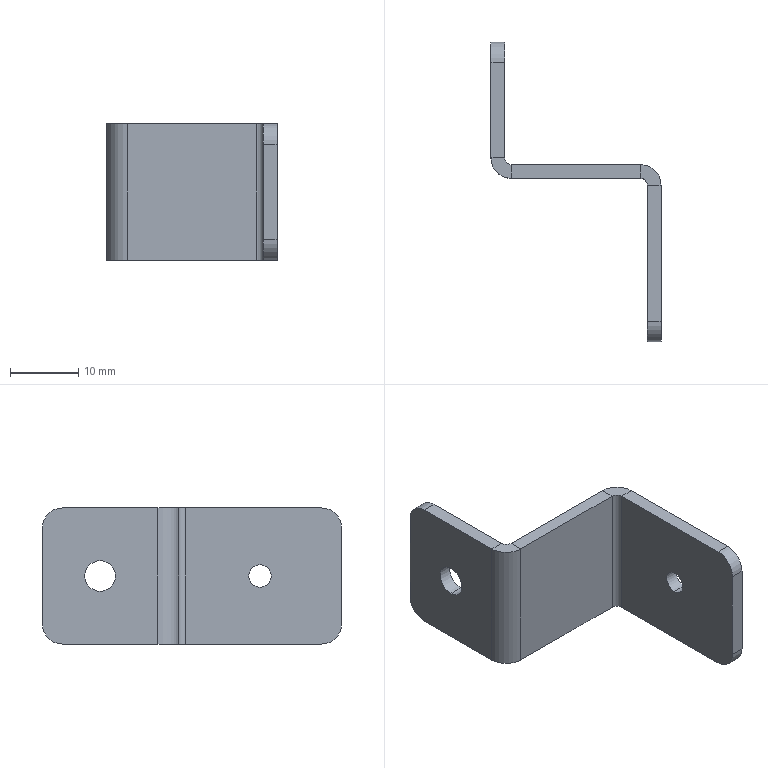Part | NX | features BREP 1 | 1 solid | 30 faces | box 25 x 44 x 20 mm | volume 2547 mm3 | plane 18 | cylinder 12 | commonest cylinder face diameters 6 x6 2 x2 3.3 x2 4.5 x2
STEP:
#1=CARTESIAN_POINT('',(23.,-12.,1.65));
#2=VERTEX_POINT('',#1);
#3=CARTESIAN_POINT('',(25.,-12.,1.65));
#4=VERTEX_POINT('',#3);
#5=CARTESIAN_POINT('',(25.,-12.,1.65));
#6=DIRECTION('',(1.,0.,0.));
#7=VECTOR('',#6,1000.);
#8=LINE('',#5,#7);
#9=EDGE_CURVE('',#2,#4,#8,.T.);
#10=ORIENTED_EDGE('',*,*,#9,.F.);
#11=CARTESIAN_POINT('',(23.,-12.,-1.65));
#12=VERTEX_POINT('',#11);
#13=CARTESIAN_POINT('',(23.,-12.,0.));
#14=DIRECTION('',(-1.,0.,0.));
#15=DIRECTION('',(0.,-1.,0.));
#16=AXIS2_PLACEMENT_3D('',#13,#14,#15);
#17=CIRCLE('',#16,1.65);
#18=EDGE_CURVE('',#2,#12,#17,.T.);
#19=ORIENTED_EDGE('',*,*,#18,.T.);
#20=CARTESIAN_POINT('',(25.,-12.,-1.65));
#21=VERTEX_POINT('',#20);
#22=CARTESIAN_POINT('',(25.,-12.,-1.65));
#23=DIRECTION('',(1.,0.,0.));
#24=VECTOR('',#23,1000.);
#25=LINE('',#22,#24);
#26=EDGE_CURVE('',#12,#21,#25,.T.);
#27=ORIENTED_EDGE('',*,*,#26,.T.);
#28=CARTESIAN_POINT('',(25.,-12.,0.));
#29=DIRECTION('',(1.,0.,0.));
#30=DIRECTION('',(0.,0.,-1.));
#31=AXIS2_PLACEMENT_3D('',#28,#29,#30);
#32=CIRCLE('',#31,1.65);
#33=EDGE_CURVE('',#21,#4,#32,.T.);
#34=ORIENTED_EDGE('',*,*,#33,.T.);
#35=EDGE_LOOP('',(#10,#19,#27,#34));
#36=FACE_BOUND('',#35,.T.);
#37=CARTESIAN_POINT('',(25.,-12.,0.));
#38=DIRECTION('',(1.,0.,0.));
#39=DIRECTION('',(0.,0.,-1.));
#40=AXIS2_PLACEMENT_3D('',#37,#38,#39);
#41=CYLINDRICAL_SURFACE('',#40,1.65);
#42=ADVANCED_FACE('',(#36),#41,.F.);
#43=CARTESIAN_POINT('',(0.,11.5,-2.25));
#44=VERTEX_POINT('',#43);
#45=CARTESIAN_POINT('',(2.,11.5,-2.25));
#46=VERTEX_POINT('',#45);
#47=CARTESIAN_POINT('',(0.,11.5,-2.25));
#48=DIRECTION('',(-1.,0.,0.));
#49=VECTOR('',#48,1000.);
#50=LINE('',#47,#49);
#51=EDGE_CURVE('',#44,#46,#50,.F.);
#52=ORIENTED_EDGE('',*,*,#51,.T.);
#53=CARTESIAN_POINT('',(2.,11.5,2.25));
#54=VERTEX_POINT('',#53);
#55=CARTESIAN_POINT('',(2.,11.5,0.));
#56=DIRECTION('',(-1.,0.,0.));
#57=DIRECTION('',(0.,0.,1.));
#58=AXIS2_PLACEMENT_3D('',#55,#56,#57);
#59=CIRCLE('',#58,2.25);
#60=EDGE_CURVE('',#54,#46,#59,.T.);
#61=ORIENTED_EDGE('',*,*,#60,.F.);
#62=CARTESIAN_POINT('',(0.,11.5,2.25));
#63=VERTEX_POINT('',#62);
#64=CARTESIAN_POINT('',(0.,11.5,2.25));
#65=DIRECTION('',(-1.,0.,0.));
#66=VECTOR('',#65,1000.);
#67=LINE('',#64,#66);
#68=EDGE_CURVE('',#63,#54,#67,.F.);
#69=ORIENTED_EDGE('',*,*,#68,.F.);
#70=CARTESIAN_POINT('',(0.,11.5,0.));
#71=DIRECTION('',(-1.,0.,0.));
#72=DIRECTION('',(0.,0.,1.));
#73=AXIS2_PLACEMENT_3D('',#70,#71,#72);
#74=CIRCLE('',#73,2.25);
#75=EDGE_CURVE('',#63,#44,#74,.T.);
#76=ORIENTED_EDGE('',*,*,#75,.T.);
#77=EDGE_LOOP('',(#52,#61,#69,#76));
#78=FACE_BOUND('',#77,.T.);
#79=CARTESIAN_POINT('',(0.,11.5,0.));
#80=DIRECTION('',(-1.,0.,0.));
#81=DIRECTION('',(0.,0.,1.));
#82=AXIS2_PLACEMENT_3D('',#79,#80,#81);
#83=CYLINDRICAL_SURFACE('',#82,2.25);
#84=ADVANCED_FACE('',(#78),#83,.F.);
#85=CARTESIAN_POINT('',(25.,-24.,-7.));
#86=VERTEX_POINT('',#85);
#87=CARTESIAN_POINT('',(25.,-21.,-10.));
#88=VERTEX_POINT('',#87);
#89=CARTESIAN_POINT('',(25.,-21.,-7.));
#90=DIRECTION('',(1.,0.,0.));
#91=DIRECTION('',(0.,-1.,0.));
#92=AXIS2_PLACEMENT_3D('',#89,#90,#91);
#93=CIRCLE('',#92,3.);
#94=EDGE_CURVE('',#86,#88,#93,.T.);
#95=ORIENTED_EDGE('',*,*,#94,.F.);
#96=CARTESIAN_POINT('',(23.,-24.,-7.));
#97=VERTEX_POINT('',#96);
#98=CARTESIAN_POINT('',(25.,-24.,-7.));
#99=DIRECTION('',(1.,0.,0.));
#100=VECTOR('',#99,1000.);
#101=LINE('',#98,#100);
#102=EDGE_CURVE('',#97,#86,#101,.T.);
#103=ORIENTED_EDGE('',*,*,#102,.F.);
#104=CARTESIAN_POINT('',(23.,-21.,-10.));
#105=VERTEX_POINT('',#104);
#106=CARTESIAN_POINT('',(23.,-21.,-7.));
#107=DIRECTION('',(-1.,0.,0.));
#108=DIRECTION('',(0.,-1.,0.));
#109=AXIS2_PLACEMENT_3D('',#106,#107,#108);
#110=CIRCLE('',#109,3.);
#111=EDGE_CURVE('',#105,#97,#110,.T.);
#112=ORIENTED_EDGE('',*,*,#111,.F.);
#113=CARTESIAN_POINT('',(22.,-21.,-10.));
#114=DIRECTION('',(-1.,0.,0.));
#115=VECTOR('',#114,1000.);
#116=LINE('',#113,#115);
#117=EDGE_CURVE('',#88,#105,#116,.T.);
#118=ORIENTED_EDGE('',*,*,#117,.F.);
#119=EDGE_LOOP('',(#95,#103,#112,#118));
#120=FACE_BOUND('',#119,.T.);
#121=CARTESIAN_POINT('',(22.,-21.,-7.));
#122=DIRECTION('',(-1.,0.,0.));
#123=DIRECTION('',(0.,0.,1.));
#124=AXIS2_PLACEMENT_3D('',#121,#122,#123);
#125=CYLINDRICAL_SURFACE('',#124,3.);
#126=ADVANCED_FACE('',(#120),#125,.T.);
#127=CARTESIAN_POINT('',(25.,-21.,10.));
#128=VERTEX_POINT('',#127);
#129=CARTESIAN_POINT('',(25.,-24.,7.));
#130=VERTEX_POINT('',#129);
#131=CARTESIAN_POINT('',(25.,-21.,7.));
#132=DIRECTION('',(1.,0.,0.));
#133=DIRECTION('',(0.,-1.,0.));
#134=AXIS2_PLACEMENT_3D('',#131,#132,#133);
#135=CIRCLE('',#134,3.);
#136=EDGE_CURVE('',#128,#130,#135,.T.);
#137=ORIENTED_EDGE('',*,*,#136,.F.);
#138=CARTESIAN_POINT('',(23.,-21.,10.));
#139=VERTEX_POINT('',#138);
#140=CARTESIAN_POINT('',(3.,-21.,10.));
#141=DIRECTION('',(1.,0.,0.));
#142=VECTOR('',#141,1000.);
#143=LINE('',#140,#142);
#144=EDGE_CURVE('',#139,#128,#143,.T.);
#145=ORIENTED_EDGE('',*,*,#144,.F.);
#146=CARTESIAN_POINT('',(23.,-24.,7.));
#147=VERTEX_POINT('',#146);
#148=CARTESIAN_POINT('',(23.,-21.,7.));
#149=DIRECTION('',(-1.,0.,0.));
#150=DIRECTION('',(0.,-1.,0.));
#151=AXIS2_PLACEMENT_3D('',#148,#149,#150);
#152=CIRCLE('',#151,3.);
#153=EDGE_CURVE('',#147,#139,#152,.T.);
#154=ORIENTED_EDGE('',*,*,#153,.F.);
#155=CARTESIAN_POINT('',(25.,-24.,7.));
#156=DIRECTION('',(-1.,0.,0.));
#157=VECTOR('',#156,1000.);
#158=LINE('',#155,#157);
#159=EDGE_CURVE('',#130,#147,#158,.T.);
#160=ORIENTED_EDGE('',*,*,#159,.F.);
#161=EDGE_LOOP('',(#137,#145,#154,#160));
#162=FACE_BOUND('',#161,.T.);
#163=CARTESIAN_POINT('',(25.,-21.,7.));
#164=DIRECTION('',(-1.,0.,0.));
#165=DIRECTION('',(0.,0.,1.));
#166=AXIS2_PLACEMENT_3D('',#163,#164,#165);
#167=CYLINDRICAL_SURFACE('',#166,3.);
#168=ADVANCED_FACE('',(#162),#167,.T.);
#169=CARTESIAN_POINT('',(0.,20.,-7.));
#170=VERTEX_POINT('',#169);
#171=CARTESIAN_POINT('',(0.,17.,-10.));
#172=VERTEX_POINT('',#171);
#173=CARTESIAN_POINT('',(0.,17.,-7.));
#174=DIRECTION('',(-1.,0.,0.));
#175=DIRECTION('',(0.,0.,1.));
#176=AXIS2_PLACEMENT_3D('',#173,#174,#175);
#177=CIRCLE('',#176,3.);
#178=EDGE_CURVE('',#170,#172,#177,.T.);
#179=ORIENTED_EDGE('',*,*,#178,.F.);
#180=CARTESIAN_POINT('',(2.,20.,-7.));
#181=VERTEX_POINT('',#180);
#182=CARTESIAN_POINT('',(0.,20.,-7.));
#183=DIRECTION('',(-1.,0.,0.));
#184=VECTOR('',#183,1000.);
#185=LINE('',#182,#184);
#186=EDGE_CURVE('',#181,#170,#185,.T.);
#187=ORIENTED_EDGE('',*,*,#186,.F.);
#188=CARTESIAN_POINT('',(2.,17.,-10.));
#189=VERTEX_POINT('',#188);
#190=CARTESIAN_POINT('',(2.,17.,-7.));
#191=DIRECTION('',(1.,0.,0.));
#192=DIRECTION('',(0.,0.,1.));
#193=AXIS2_PLACEMENT_3D('',#190,#191,#192);
#194=CIRCLE('',#193,3.);
#195=EDGE_CURVE('',#189,#181,#194,.T.);
#196=ORIENTED_EDGE('',*,*,#195,.F.);
#197=CARTESIAN_POINT('',(2.,17.,-10.));
#198=DIRECTION('',(1.,0.,0.));
#199=VECTOR('',#198,1000.);
#200=LINE('',#197,#199);
#201=EDGE_CURVE('',#172,#189,#200,.T.);
#202=ORIENTED_EDGE('',*,*,#201,.F.);
#203=EDGE_LOOP('',(#179,#187,#196,#202));
#204=FACE_BOUND('',#203,.T.);
#205=CARTESIAN_POINT('',(3.,17.,-7.));
#206=DIRECTION('',(-1.,0.,0.));
#207=DIRECTION('',(0.,0.,1.));
#208=AXIS2_PLACEMENT_3D('',#205,#206,#207);
#209=CYLINDRICAL_SURFACE('',#208,3.);
#210=ADVANCED_FACE('',(#204),#209,.T.);
#211=CARTESIAN_POINT('',(0.,17.,10.));
#212=VERTEX_POINT('',#211);
#213=CARTESIAN_POINT('',(0.,20.,7.));
#214=VERTEX_POINT('',#213);
#215=CARTESIAN_POINT('',(0.,17.,7.));
#216=DIRECTION('',(-1.,0.,0.));
#217=DIRECTION('',(0.,0.,1.));
#218=AXIS2_PLACEMENT_3D('',#215,#216,#217);
#219=CIRCLE('',#218,3.);
#220=EDGE_CURVE('',#212,#214,#219,.T.);
#221=ORIENTED_EDGE('',*,*,#220,.F.);
#222=CARTESIAN_POINT('',(2.,17.,10.));
#223=VERTEX_POINT('',#222);
#224=CARTESIAN_POINT('',(3.,17.,10.));
#225=DIRECTION('',(-1.,0.,0.));
#226=VECTOR('',#225,1000.);
#227=LINE('',#224,#226);
#228=EDGE_CURVE('',#223,#212,#227,.T.);
#229=ORIENTED_EDGE('',*,*,#228,.F.);
#230=CARTESIAN_POINT('',(2.,20.,7.));
#231=VERTEX_POINT('',#230);
#232=CARTESIAN_POINT('',(2.,17.,7.));
#233=DIRECTION('',(1.,0.,0.));
#234=DIRECTION('',(0.,0.,1.));
#235=AXIS2_PLACEMENT_3D('',#232,#233,#234);
#236=CIRCLE('',#235,3.);
#237=EDGE_CURVE('',#231,#223,#236,.T.);
#238=ORIENTED_EDGE('',*,*,#237,.F.);
#239=CARTESIAN_POINT('',(0.,20.,7.));
#240=DIRECTION('',(1.,0.,0.));
#241=VECTOR('',#240,1000.);
#242=LINE('',#239,#241);
#243=EDGE_CURVE('',#214,#231,#242,.T.);
#244=ORIENTED_EDGE('',*,*,#243,.F.);
#245=EDGE_LOOP('',(#221,#229,#238,#244));
#246=FACE_BOUND('',#245,.T.);
#247=CARTESIAN_POINT('',(0.,17.,7.));
#248=DIRECTION('',(1.,0.,0.));
#249=DIRECTION('',(0.,0.,-1.));
#250=AXIS2_PLACEMENT_3D('',#247,#248,#249);
#251=CYLINDRICAL_SURFACE('',#250,3.);
#252=ADVANCED_FACE('',(#246),#251,.T.);
#253=CARTESIAN_POINT('',(0.,3.,-10.));
#254=VERTEX_POINT('',#253);
#255=CARTESIAN_POINT('',(0.,0.,-10.));
#256=DIRECTION('',(0.,1.,0.));
#257=VECTOR('',#256,1000.);
#258=LINE('',#255,#257);
#259=EDGE_CURVE('',#254,#172,#258,.T.);
#260=ORIENTED_EDGE('',*,*,#259,.T.);
#261=ORIENTED_EDGE('',*,*,#201,.T.);
#262=CARTESIAN_POINT('',(2.,3.,-10.));
#263=VERTEX_POINT('',#262);
#264=CARTESIAN_POINT('',(2.,0.,-10.));
#265=DIRECTION('',(0.,1.,0.));
#266=VECTOR('',#265,1000.);
#267=LINE('',#264,#266);
#268=EDGE_CURVE('',#263,#189,#267,.T.);
#269=ORIENTED_EDGE('',*,*,#268,.F.);
#270=CARTESIAN_POINT('',(2.,3.,-10.));
#271=DIRECTION('',(-1.,0.,0.));
#272=VECTOR('',#271,1000.);
#273=LINE('',#270,#272);
#274=EDGE_CURVE('',#263,#254,#273,.T.);
#275=ORIENTED_EDGE('',*,*,#274,.T.);
#276=EDGE_LOOP('',(#260,#261,#269,#275));
#277=FACE_BOUND('',#276,.T.);
#278=CARTESIAN_POINT('',(3.,3.,-10.));
#279=DIRECTION('',(0.,0.,1.));
#280=DIRECTION('',(1.,0.,0.));
#281=AXIS2_PLACEMENT_3D('',#278,#279,#280);
#282=PLANE('',#281);
#283=ADVANCED_FACE('',(#277),#282,.F.);
#284=CARTESIAN_POINT('',(23.,-1.,10.));
#285=VERTEX_POINT('',#284);
#286=CARTESIAN_POINT('',(23.,0.,10.));
#287=DIRECTION('',(0.,1.,0.));
#288=VECTOR('',#287,1000.);
#289=LINE('',#286,#288);
#290=EDGE_CURVE('',#139,#285,#289,.T.);
#291=ORIENTED_EDGE('',*,*,#290,.F.);
#292=ORIENTED_EDGE('',*,*,#144,.T.);
#293=CARTESIAN_POINT('',(25.,-1.,10.));
#294=VERTEX_POINT('',#293);
#295=CARTESIAN_POINT('',(25.,0.,10.));
#296=DIRECTION('',(0.,1.,0.));
#297=VECTOR('',#296,1000.);
#298=LINE('',#295,#297);
#299=EDGE_CURVE('',#128,#294,#298,.T.);
#300=ORIENTED_EDGE('',*,*,#299,.T.);
#301=CARTESIAN_POINT('',(25.,-1.,10.));
#302=DIRECTION('',(-1.,0.,0.));
#303=VECTOR('',#302,1000.);
#304=LINE('',#301,#303);
#305=EDGE_CURVE('',#294,#285,#304,.T.);
#306=ORIENTED_EDGE('',*,*,#305,.T.);
#307=EDGE_LOOP('',(#291,#292,#300,#306));
#308=FACE_BOUND('',#307,.T.);
#309=CARTESIAN_POINT('',(3.,3.,10.));
#310=DIRECTION('',(0.,0.,1.));
#311=DIRECTION('',(1.,0.,0.));
#312=AXIS2_PLACEMENT_3D('',#309,#310,#311);
#313=PLANE('',#312);
#314=ADVANCED_FACE('',(#308),#313,.T.);
#315=CARTESIAN_POINT('',(3.,2.,-10.));
#316=VERTEX_POINT('',#315);
#317=CARTESIAN_POINT('',(3.,3.,-10.));
#318=DIRECTION('',(0.,0.,-1.));
#319=DIRECTION('',(1.,0.,0.));
#320=AXIS2_PLACEMENT_3D('',#317,#318,#319);
#321=CIRCLE('',#320,1.);
#322=EDGE_CURVE('',#316,#263,#321,.T.);
#323=ORIENTED_EDGE('',*,*,#322,.T.);
#324=CARTESIAN_POINT('',(2.,3.,10.));
#325=VERTEX_POINT('',#324);
#326=CARTESIAN_POINT('',(2.,3.,10.));
#327=DIRECTION('',(0.,0.,-1.));
#328=VECTOR('',#327,1000.);
#329=LINE('',#326,#328);
#330=EDGE_CURVE('',#325,#263,#329,.T.);
#331=ORIENTED_EDGE('',*,*,#330,.F.);
#332=CARTESIAN_POINT('',(3.,2.,10.));
#333=VERTEX_POINT('',#332);
#334=CARTESIAN_POINT('',(3.,3.,10.));
#335=DIRECTION('',(0.,0.,-1.));
#336=DIRECTION('',(1.,0.,0.));
#337=AXIS2_PLACEMENT_3D('',#334,#335,#336);
#338=CIRCLE('',#337,1.);
#339=EDGE_CURVE('',#333,#325,#338,.T.);
#340=ORIENTED_EDGE('',*,*,#339,.F.);
#341=CARTESIAN_POINT('',(3.,2.,10.));
#342=DIRECTION('',(0.,0.,-1.));
#343=VECTOR('',#342,1000.);
#344=LINE('',#341,#343);
#345=EDGE_CURVE('',#333,#316,#344,.T.);
#346=ORIENTED_EDGE('',*,*,#345,.T.);
#347=EDGE_LOOP('',(#323,#331,#340,#346));
#348=FACE_BOUND('',#347,.T.);
#349=CARTESIAN_POINT('',(3.,3.,10.));
#350=DIRECTION('',(0.,0.,-1.));
#351=DIRECTION('',(-1.,0.,0.));
#352=AXIS2_PLACEMENT_3D('',#349,#350,#351);
#353=CYLINDRICAL_SURFACE('',#352,1.);
#354=ADVANCED_FACE('',(#348),#353,.F.);
#355=CARTESIAN_POINT('',(22.,2.,-10.));
#356=VERTEX_POINT('',#355);
#357=CARTESIAN_POINT('',(0.,2.,-10.));
#358=DIRECTION('',(-1.,0.,0.));
#359=VECTOR('',#358,1000.);
#360=LINE('',#357,#359);
#361=EDGE_CURVE('',#356,#316,#360,.T.);
#362=ORIENTED_EDGE('',*,*,#361,.T.);
#363=ORIENTED_EDGE('',*,*,#345,.F.);
#364=CARTESIAN_POINT('',(22.,2.,10.));
#365=VERTEX_POINT('',#364);
#366=CARTESIAN_POINT('',(0.,2.,10.));
#367=DIRECTION('',(-1.,0.,0.));
#368=VECTOR('',#367,1000.);
#369=LINE('',#366,#368);
#370=EDGE_CURVE('',#365,#333,#369,.T.);
#371=ORIENTED_EDGE('',*,*,#370,.F.);
#372=CARTESIAN_POINT('',(22.,2.,10.));
#373=DIRECTION('',(0.,0.,-1.));
#374=VECTOR('',#373,1000.);
#375=LINE('',#372,#374);
#376=EDGE_CURVE('',#365,#356,#375,.T.);
#377=ORIENTED_EDGE('',*,*,#376,.T.);
#378=EDGE_LOOP('',(#362,#363,#371,#377));
#379=FACE_BOUND('',#378,.T.);
#380=CARTESIAN_POINT('',(0.,2.,10.));
#381=DIRECTION('',(0.,-1.,0.));
#382=DIRECTION('',(0.,0.,-1.));
#383=AXIS2_PLACEMENT_3D('',#380,#381,#382);
#384=PLANE('',#383);
#385=ADVANCED_FACE('',(#379),#384,.F.);
#386=CARTESIAN_POINT('',(25.,-1.,-10.));
#387=VERTEX_POINT('',#386);
#388=CARTESIAN_POINT('',(22.,-1.,-10.));
#389=DIRECTION('',(0.,0.,1.));
#390=DIRECTION('',(1.,0.,0.));
#391=AXIS2_PLACEMENT_3D('',#388,#389,#390);
#392=CIRCLE('',#391,3.);
#393=EDGE_CURVE('',#387,#356,#392,.T.);
#394=ORIENTED_EDGE('',*,*,#393,.T.);
#395=ORIENTED_EDGE('',*,*,#376,.F.);
#396=CARTESIAN_POINT('',(22.,-1.,10.));
#397=DIRECTION('',(0.,0.,1.));
#398=DIRECTION('',(1.,0.,0.));
#399=AXIS2_PLACEMENT_3D('',#396,#397,#398);
#400=CIRCLE('',#399,3.);
#401=EDGE_CURVE('',#294,#365,#400,.T.);
#402=ORIENTED_EDGE('',*,*,#401,.F.);
#403=CARTESIAN_POINT('',(25.,-1.,10.));
#404=DIRECTION('',(0.,0.,-1.));
#405=VECTOR('',#404,1000.);
#406=LINE('',#403,#405);
#407=EDGE_CURVE('',#294,#387,#406,.T.);
#408=ORIENTED_EDGE('',*,*,#407,.T.);
#409=EDGE_LOOP('',(#394,#395,#402,#408));
#410=FACE_BOUND('',#409,.T.);
#411=CARTESIAN_POINT('',(22.,-1.,10.));
#412=DIRECTION('',(0.,0.,-1.));
#413=DIRECTION('',(-1.,0.,0.));
#414=AXIS2_PLACEMENT_3D('',#411,#412,#413);
#415=CYLINDRICAL_SURFACE('',#414,3.);
#416=ADVANCED_FACE('',(#410),#415,.T.);
#417=ORIENTED_EDGE('',*,*,#299,.F.);
#418=ORIENTED_EDGE('',*,*,#136,.T.);
#419=CARTESIAN_POINT('',(25.,-24.,10.));
#420=DIRECTION('',(0.,0.,-1.));
#421=VECTOR('',#420,1000.);
#422=LINE('',#419,#421);
#423=EDGE_CURVE('',#130,#86,#422,.T.);
#424=ORIENTED_EDGE('',*,*,#423,.T.);
#425=ORIENTED_EDGE('',*,*,#94,.T.);
#426=CARTESIAN_POINT('',(25.,0.,-10.));
#427=DIRECTION('',(0.,1.,0.));
#428=VECTOR('',#427,1000.);
#429=LINE('',#426,#428);
#430=EDGE_CURVE('',#88,#387,#429,.T.);
#431=ORIENTED_EDGE('',*,*,#430,.T.);
#432=ORIENTED_EDGE('',*,*,#407,.F.);
#433=EDGE_LOOP('',(#417,#418,#424,#425,#431,#432));
#434=FACE_BOUND('',#433,.T.);
#435=ORIENTED_EDGE('',*,*,#33,.F.);
#436=CARTESIAN_POINT('',(25.,-12.,0.));
#437=DIRECTION('',(1.,0.,0.));
#438=DIRECTION('',(0.,0.,-1.));
#439=AXIS2_PLACEMENT_3D('',#436,#437,#438);
#440=CIRCLE('',#439,1.65);
#441=EDGE_CURVE('',#4,#21,#440,.T.);
#442=ORIENTED_EDGE('',*,*,#441,.F.);
#443=EDGE_LOOP('',(#435,#442));
#444=FACE_BOUND('',#443,.T.);
#445=CARTESIAN_POINT('',(25.,0.,10.));
#446=DIRECTION('',(-1.,0.,0.));
#447=DIRECTION('',(0.,-1.,0.));
#448=AXIS2_PLACEMENT_3D('',#445,#446,#447);
#449=PLANE('',#448);
#450=ADVANCED_FACE('',(#434,#444),#449,.F.);
#451=ORIENTED_EDGE('',*,*,#423,.F.);
#452=ORIENTED_EDGE('',*,*,#159,.T.);
#453=CARTESIAN_POINT('',(23.,-24.,10.));
#454=DIRECTION('',(0.,0.,-1.));
#455=VECTOR('',#454,1000.);
#456=LINE('',#453,#455);
#457=EDGE_CURVE('',#147,#97,#456,.T.);
#458=ORIENTED_EDGE('',*,*,#457,.T.);
#459=ORIENTED_EDGE('',*,*,#102,.T.);
#460=EDGE_LOOP('',(#451,#452,#458,#459));
#461=FACE_BOUND('',#460,.T.);
#462=CARTESIAN_POINT('',(25.,-24.,10.));
#463=DIRECTION('',(0.,-1.,0.));
#464=DIRECTION('',(0.,0.,-1.));
#465=AXIS2_PLACEMENT_3D('',#462,#463,#464);
#466=PLANE('',#465);
#467=ADVANCED_FACE('',(#461),#466,.T.);
#468=ORIENTED_EDGE('',*,*,#457,.F.);
#469=ORIENTED_EDGE('',*,*,#153,.T.);
#470=ORIENTED_EDGE('',*,*,#290,.T.);
#471=CARTESIAN_POINT('',(23.,-1.,-10.));
#472=VERTEX_POINT('',#471);
#473=CARTESIAN_POINT('',(23.,-1.,10.));
#474=DIRECTION('',(0.,0.,-1.));
#475=VECTOR('',#474,1000.);
#476=LINE('',#473,#475);
#477=EDGE_CURVE('',#285,#472,#476,.T.);
#478=ORIENTED_EDGE('',*,*,#477,.T.);
#479=CARTESIAN_POINT('',(23.,0.,-10.));
#480=DIRECTION('',(0.,1.,0.));
#481=VECTOR('',#480,1000.);
#482=LINE('',#479,#481);
#483=EDGE_CURVE('',#105,#472,#482,.T.);
#484=ORIENTED_EDGE('',*,*,#483,.F.);
#485=ORIENTED_EDGE('',*,*,#111,.T.);
#486=EDGE_LOOP('',(#468,#469,#470,#478,#484,#485));
#487=FACE_BOUND('',#486,.T.);
#488=CARTESIAN_POINT('',(23.,-12.,0.));
#489=DIRECTION('',(-1.,0.,0.));
#490=DIRECTION('',(0.,-1.,0.));
#491=AXIS2_PLACEMENT_3D('',#488,#489,#490);
#492=CIRCLE('',#491,1.65);
#493=EDGE_CURVE('',#12,#2,#492,.T.);
#494=ORIENTED_EDGE('',*,*,#493,.F.);
#495=ORIENTED_EDGE('',*,*,#18,.F.);
#496=EDGE_LOOP('',(#494,#495));
#497=FACE_BOUND('',#496,.T.);
#498=CARTESIAN_POINT('',(23.,0.,10.));
#499=DIRECTION('',(-1.,0.,0.));
#500=DIRECTION('',(0.,-1.,0.));
#501=AXIS2_PLACEMENT_3D('',#498,#499,#500);
#502=PLANE('',#501);
#503=ADVANCED_FACE('',(#487,#497),#502,.T.);
#504=CARTESIAN_POINT('',(22.,0.,-10.));
#505=VERTEX_POINT('',#504);
#506=CARTESIAN_POINT('',(22.,-1.,-10.));
#507=DIRECTION('',(0.,0.,1.));
#508=DIRECTION('',(-1.,0.,0.));
#509=AXIS2_PLACEMENT_3D('',#506,#507,#508);
#510=CIRCLE('',#509,1.);
#511=EDGE_CURVE('',#472,#505,#510,.T.);
#512=ORIENTED_EDGE('',*,*,#511,.F.);
#513=ORIENTED_EDGE('',*,*,#477,.F.);
#514=CARTESIAN_POINT('',(22.,0.,10.));
#515=VERTEX_POINT('',#514);
#516=CARTESIAN_POINT('',(22.,-1.,10.));
#517=DIRECTION('',(0.,0.,1.));
#518=DIRECTION('',(-1.,0.,0.));
#519=AXIS2_PLACEMENT_3D('',#516,#517,#518);
#520=CIRCLE('',#519,1.);
#521=EDGE_CURVE('',#285,#515,#520,.T.);
#522=ORIENTED_EDGE('',*,*,#521,.T.);
#523=CARTESIAN_POINT('',(22.,0.,10.));
#524=DIRECTION('',(0.,0.,-1.));
#525=VECTOR('',#524,1000.);
#526=LINE('',#523,#525);
#527=EDGE_CURVE('',#515,#505,#526,.T.);
#528=ORIENTED_EDGE('',*,*,#527,.T.);
#529=EDGE_LOOP('',(#512,#513,#522,#528));
#530=FACE_BOUND('',#529,.T.);
#531=CARTESIAN_POINT('',(22.,-1.,10.));
#532=DIRECTION('',(0.,0.,-1.));
#533=DIRECTION('',(-1.,0.,0.));
#534=AXIS2_PLACEMENT_3D('',#531,#532,#533);
#535=CYLINDRICAL_SURFACE('',#534,1.);
#536=ADVANCED_FACE('',(#530),#535,.F.);
#537=CARTESIAN_POINT('',(3.,0.,-10.));
#538=VERTEX_POINT('',#537);
#539=CARTESIAN_POINT('',(0.,0.,-10.));
#540=DIRECTION('',(-1.,0.,0.));
#541=VECTOR('',#540,1000.);
#542=LINE('',#539,#541);
#543=EDGE_CURVE('',#505,#538,#542,.T.);
#544=ORIENTED_EDGE('',*,*,#543,.F.);
#545=ORIENTED_EDGE('',*,*,#527,.F.);
#546=CARTESIAN_POINT('',(3.,0.,10.));
#547=VERTEX_POINT('',#546);
#548=CARTESIAN_POINT('',(0.,0.,10.));
#549=DIRECTION('',(-1.,0.,0.));
#550=VECTOR('',#549,1000.);
#551=LINE('',#548,#550);
#552=EDGE_CURVE('',#515,#547,#551,.T.);
#553=ORIENTED_EDGE('',*,*,#552,.T.);
#554=CARTESIAN_POINT('',(3.,0.,10.));
#555=DIRECTION('',(0.,0.,-1.));
#556=VECTOR('',#555,1000.);
#557=LINE('',#554,#556);
#558=EDGE_CURVE('',#547,#538,#557,.T.);
#559=ORIENTED_EDGE('',*,*,#558,.T.);
#560=EDGE_LOOP('',(#544,#545,#553,#559));
#561=FACE_BOUND('',#560,.T.);
#562=CARTESIAN_POINT('',(0.,0.,10.));
#563=DIRECTION('',(0.,-1.,0.));
#564=DIRECTION('',(0.,0.,-1.));
#565=AXIS2_PLACEMENT_3D('',#562,#563,#564);
#566=PLANE('',#565);
#567=ADVANCED_FACE('',(#561),#566,.T.);
#568=CARTESIAN_POINT('',(3.,3.,-10.));
#569=DIRECTION('',(0.,0.,-1.));
#570=DIRECTION('',(1.,0.,0.));
#571=AXIS2_PLACEMENT_3D('',#568,#569,#570);
#572=CIRCLE('',#571,3.);
#573=EDGE_CURVE('',#538,#254,#572,.T.);
#574=ORIENTED_EDGE('',*,*,#573,.F.);
#575=ORIENTED_EDGE('',*,*,#558,.F.);
#576=CARTESIAN_POINT('',(0.,3.,10.));
#577=VERTEX_POINT('',#576);
#578=CARTESIAN_POINT('',(3.,3.,10.));
#579=DIRECTION('',(0.,0.,-1.));
#580=DIRECTION('',(1.,0.,0.));
#581=AXIS2_PLACEMENT_3D('',#578,#579,#580);
#582=CIRCLE('',#581,3.);
#583=EDGE_CURVE('',#547,#577,#582,.T.);
#584=ORIENTED_EDGE('',*,*,#583,.T.);
#585=CARTESIAN_POINT('',(0.,3.,10.));
#586=DIRECTION('',(0.,0.,-1.));
#587=VECTOR('',#586,1000.);
#588=LINE('',#585,#587);
#589=EDGE_CURVE('',#577,#254,#588,.T.);
#590=ORIENTED_EDGE('',*,*,#589,.T.);
#591=EDGE_LOOP('',(#574,#575,#584,#590));
#592=FACE_BOUND('',#591,.T.);
#593=CARTESIAN_POINT('',(3.,3.,10.));
#594=DIRECTION('',(0.,0.,-1.));
#595=DIRECTION('',(-1.,0.,0.));
#596=AXIS2_PLACEMENT_3D('',#593,#594,#595);
#597=CYLINDRICAL_SURFACE('',#596,3.);
#598=ADVANCED_FACE('',(#592),#597,.T.);
#599=CARTESIAN_POINT('',(0.,0.,10.));
#600=DIRECTION('',(0.,1.,0.));
#601=VECTOR('',#600,1000.);
#602=LINE('',#599,#601);
#603=EDGE_CURVE('',#577,#212,#602,.T.);
#604=ORIENTED_EDGE('',*,*,#603,.T.);
#605=ORIENTED_EDGE('',*,*,#220,.T.);
#606=CARTESIAN_POINT('',(0.,20.,10.));
#607=DIRECTION('',(0.,0.,-1.));
#608=VECTOR('',#607,1000.);
#609=LINE('',#606,#608);
#610=EDGE_CURVE('',#214,#170,#609,.T.);
#611=ORIENTED_EDGE('',*,*,#610,.T.);
#612=ORIENTED_EDGE('',*,*,#178,.T.);
#613=ORIENTED_EDGE('',*,*,#259,.F.);
#614=ORIENTED_EDGE('',*,*,#589,.F.);
#615=EDGE_LOOP('',(#604,#605,#611,#612,#613,#614));
#616=FACE_BOUND('',#615,.T.);
#617=ORIENTED_EDGE('',*,*,#75,.F.);
#618=CARTESIAN_POINT('',(0.,11.5,0.));
#619=DIRECTION('',(-1.,0.,0.));
#620=DIRECTION('',(0.,0.,1.));
#621=AXIS2_PLACEMENT_3D('',#618,#619,#620);
#622=CIRCLE('',#621,2.25);
#623=EDGE_CURVE('',#44,#63,#622,.T.);
#624=ORIENTED_EDGE('',*,*,#623,.F.);
#625=EDGE_LOOP('',(#617,#624));
#626=FACE_BOUND('',#625,.T.);
#627=CARTESIAN_POINT('',(0.,0.,10.));
#628=DIRECTION('',(-1.,0.,0.));
#629=DIRECTION('',(0.,0.,1.));
#630=AXIS2_PLACEMENT_3D('',#627,#628,#629);
#631=PLANE('',#630);
#632=ADVANCED_FACE('',(#616,#626),#631,.T.);
#633=ORIENTED_EDGE('',*,*,#610,.F.);
#634=ORIENTED_EDGE('',*,*,#243,.T.);
#635=CARTESIAN_POINT('',(2.,20.,10.));
#636=DIRECTION('',(0.,0.,-1.));
#637=VECTOR('',#636,1000.);
#638=LINE('',#635,#637);
#639=EDGE_CURVE('',#231,#181,#638,.T.);
#640=ORIENTED_EDGE('',*,*,#639,.T.);
#641=ORIENTED_EDGE('',*,*,#186,.T.);
#642=EDGE_LOOP('',(#633,#634,#640,#641));
#643=FACE_BOUND('',#642,.T.);
#644=CARTESIAN_POINT('',(0.,20.,10.));
#645=DIRECTION('',(0.,1.,0.));
#646=DIRECTION('',(0.,0.,1.));
#647=AXIS2_PLACEMENT_3D('',#644,#645,#646);
#648=PLANE('',#647);
#649=ADVANCED_FACE('',(#643),#648,.T.);
#650=ORIENTED_EDGE('',*,*,#639,.F.);
#651=ORIENTED_EDGE('',*,*,#237,.T.);
#652=CARTESIAN_POINT('',(2.,0.,10.));
#653=DIRECTION('',(0.,1.,0.));
#654=VECTOR('',#653,1000.);
#655=LINE('',#652,#654);
#656=EDGE_CURVE('',#325,#223,#655,.T.);
#657=ORIENTED_EDGE('',*,*,#656,.F.);
#658=ORIENTED_EDGE('',*,*,#330,.T.);
#659=ORIENTED_EDGE('',*,*,#268,.T.);
#660=ORIENTED_EDGE('',*,*,#195,.T.);
#661=EDGE_LOOP('',(#650,#651,#657,#658,#659,#660));
#662=FACE_BOUND('',#661,.T.);
#663=ORIENTED_EDGE('',*,*,#60,.T.);
#664=CARTESIAN_POINT('',(2.,11.5,0.));
#665=DIRECTION('',(-1.,0.,0.));
#666=DIRECTION('',(0.,0.,1.));
#667=AXIS2_PLACEMENT_3D('',#664,#665,#666);
#668=CIRCLE('',#667,2.25);
#669=EDGE_CURVE('',#46,#54,#668,.T.);
#670=ORIENTED_EDGE('',*,*,#669,.T.);
#671=EDGE_LOOP('',(#663,#670));
#672=FACE_BOUND('',#671,.T.);
#673=CARTESIAN_POINT('',(2.,0.,10.));
#674=DIRECTION('',(-1.,0.,0.));
#675=DIRECTION('',(0.,0.,1.));
#676=AXIS2_PLACEMENT_3D('',#673,#674,#675);
#677=PLANE('',#676);
#678=ADVANCED_FACE('',(#662,#672),#677,.F.);
#679=ORIENTED_EDGE('',*,*,#543,.T.);
#680=CARTESIAN_POINT('',(3.,0.,-10.));
#681=DIRECTION('',(0.,1.,0.));
#682=VECTOR('',#681,1000.);
#683=LINE('',#680,#682);
#684=EDGE_CURVE('',#538,#316,#683,.T.);
#685=ORIENTED_EDGE('',*,*,#684,.T.);
#686=ORIENTED_EDGE('',*,*,#361,.F.);
#687=CARTESIAN_POINT('',(22.,2.,-10.));
#688=DIRECTION('',(0.,-1.,0.));
#689=VECTOR('',#688,1000.);
#690=LINE('',#687,#689);
#691=EDGE_CURVE('',#356,#505,#690,.T.);
#692=ORIENTED_EDGE('',*,*,#691,.T.);
#693=EDGE_LOOP('',(#679,#685,#686,#692));
#694=FACE_BOUND('',#693,.T.);
#695=CARTESIAN_POINT('',(2.,3.,-10.));
#696=DIRECTION('',(0.,0.,-1.));
#697=DIRECTION('',(-1.,0.,0.));
#698=AXIS2_PLACEMENT_3D('',#695,#696,#697);
#699=PLANE('',#698);
#700=ADVANCED_FACE('',(#694),#699,.T.);
#701=ORIENTED_EDGE('',*,*,#684,.F.);
#702=ORIENTED_EDGE('',*,*,#573,.T.);
#703=ORIENTED_EDGE('',*,*,#274,.F.);
#704=ORIENTED_EDGE('',*,*,#322,.F.);
#705=EDGE_LOOP('',(#701,#702,#703,#704));
#706=FACE_BOUND('',#705,.T.);
#707=CARTESIAN_POINT('',(3.,0.,-10.));
#708=DIRECTION('',(0.,0.,-1.));
#709=DIRECTION('',(-1.,0.,0.));
#710=AXIS2_PLACEMENT_3D('',#707,#708,#709);
#711=PLANE('',#710);
#712=ADVANCED_FACE('',(#706),#711,.T.);
#713=ORIENTED_EDGE('',*,*,#656,.T.);
#714=ORIENTED_EDGE('',*,*,#228,.T.);
#715=ORIENTED_EDGE('',*,*,#603,.F.);
#716=CARTESIAN_POINT('',(0.,3.,10.));
#717=DIRECTION('',(1.,0.,0.));
#718=VECTOR('',#717,1000.);
#719=LINE('',#716,#718);
#720=EDGE_CURVE('',#577,#325,#719,.T.);
#721=ORIENTED_EDGE('',*,*,#720,.T.);
#722=EDGE_LOOP('',(#713,#714,#715,#721));
#723=FACE_BOUND('',#722,.T.);
#724=CARTESIAN_POINT('',(3.,2.,10.));
#725=DIRECTION('',(0.,0.,1.));
#726=DIRECTION('',(1.,0.,0.));
#727=AXIS2_PLACEMENT_3D('',#724,#725,#726);
#728=PLANE('',#727);
#729=ADVANCED_FACE('',(#723),#728,.T.);
#730=ORIENTED_EDGE('',*,*,#720,.F.);
#731=ORIENTED_EDGE('',*,*,#583,.F.);
#732=CARTESIAN_POINT('',(3.,2.,10.));
#733=DIRECTION('',(0.,-1.,0.));
#734=VECTOR('',#733,1000.);
#735=LINE('',#732,#734);
#736=EDGE_CURVE('',#333,#547,#735,.T.);
#737=ORIENTED_EDGE('',*,*,#736,.F.);
#738=ORIENTED_EDGE('',*,*,#339,.T.);
#739=EDGE_LOOP('',(#730,#731,#737,#738));
#740=FACE_BOUND('',#739,.T.);
#741=CARTESIAN_POINT('',(0.,3.,10.));
#742=DIRECTION('',(0.,0.,1.));
#743=DIRECTION('',(1.,0.,0.));
#744=AXIS2_PLACEMENT_3D('',#741,#742,#743);
#745=PLANE('',#744);
#746=ADVANCED_FACE('',(#740),#745,.T.);
#747=ORIENTED_EDGE('',*,*,#430,.F.);
#748=ORIENTED_EDGE('',*,*,#117,.T.);
#749=ORIENTED_EDGE('',*,*,#483,.T.);
#750=CARTESIAN_POINT('',(23.,-1.,-10.));
#751=DIRECTION('',(1.,0.,0.));
#752=VECTOR('',#751,1000.);
#753=LINE('',#750,#752);
#754=EDGE_CURVE('',#472,#387,#753,.T.);
#755=ORIENTED_EDGE('',*,*,#754,.T.);
#756=EDGE_LOOP('',(#747,#748,#749,#755));
#757=FACE_BOUND('',#756,.T.);
#758=CARTESIAN_POINT('',(22.,2.,-10.));
#759=DIRECTION('',(0.,0.,-1.));
#760=DIRECTION('',(-1.,0.,0.));
#761=AXIS2_PLACEMENT_3D('',#758,#759,#760);
#762=PLANE('',#761);
#763=ADVANCED_FACE('',(#757),#762,.T.);
#764=ORIENTED_EDGE('',*,*,#754,.F.);
#765=ORIENTED_EDGE('',*,*,#511,.T.);
#766=ORIENTED_EDGE('',*,*,#691,.F.);
#767=ORIENTED_EDGE('',*,*,#393,.F.);
#768=EDGE_LOOP('',(#764,#765,#766,#767));
#769=FACE_BOUND('',#768,.T.);
#770=CARTESIAN_POINT('',(23.,-1.,-10.));
#771=DIRECTION('',(0.,0.,-1.));
#772=DIRECTION('',(-1.,0.,0.));
#773=AXIS2_PLACEMENT_3D('',#770,#771,#772);
#774=PLANE('',#773);
#775=ADVANCED_FACE('',(#769),#774,.T.);
#776=ORIENTED_EDGE('',*,*,#552,.F.);
#777=CARTESIAN_POINT('',(22.,0.,10.));
#778=DIRECTION('',(0.,1.,0.));
#779=VECTOR('',#778,1000.);
#780=LINE('',#777,#779);
#781=EDGE_CURVE('',#515,#365,#780,.T.);
#782=ORIENTED_EDGE('',*,*,#781,.T.);
#783=ORIENTED_EDGE('',*,*,#370,.T.);
#784=ORIENTED_EDGE('',*,*,#736,.T.);
#785=EDGE_LOOP('',(#776,#782,#783,#784));
#786=FACE_BOUND('',#785,.T.);
#787=CARTESIAN_POINT('',(25.,-1.,10.));
#788=DIRECTION('',(0.,0.,1.));
#789=DIRECTION('',(1.,0.,0.));
#790=AXIS2_PLACEMENT_3D('',#787,#788,#789);
#791=PLANE('',#790);
#792=ADVANCED_FACE('',(#786),#791,.T.);
#793=ORIENTED_EDGE('',*,*,#781,.F.);
#794=ORIENTED_EDGE('',*,*,#521,.F.);
#795=ORIENTED_EDGE('',*,*,#305,.F.);
#796=ORIENTED_EDGE('',*,*,#401,.T.);
#797=EDGE_LOOP('',(#793,#794,#795,#796));
#798=FACE_BOUND('',#797,.T.);
#799=CARTESIAN_POINT('',(22.,0.,10.));
#800=DIRECTION('',(0.,0.,1.));
#801=DIRECTION('',(1.,0.,0.));
#802=AXIS2_PLACEMENT_3D('',#799,#800,#801);
#803=PLANE('',#802);
#804=ADVANCED_FACE('',(#798),#803,.T.);
#805=ORIENTED_EDGE('',*,*,#669,.F.);
#806=ORIENTED_EDGE('',*,*,#51,.F.);
#807=ORIENTED_EDGE('',*,*,#623,.T.);
#808=ORIENTED_EDGE('',*,*,#68,.T.);
#809=EDGE_LOOP('',(#805,#806,#807,#808));
#810=FACE_BOUND('',#809,.T.);
#811=CARTESIAN_POINT('',(0.,11.5,0.));
#812=DIRECTION('',(-1.,0.,0.));
#813=DIRECTION('',(0.,0.,1.));
#814=AXIS2_PLACEMENT_3D('',#811,#812,#813);
#815=CYLINDRICAL_SURFACE('',#814,2.25);
#816=ADVANCED_FACE('',(#810),#815,.F.);
#817=ORIENTED_EDGE('',*,*,#493,.T.);
#818=ORIENTED_EDGE('',*,*,#9,.T.);
#819=ORIENTED_EDGE('',*,*,#441,.T.);
#820=ORIENTED_EDGE('',*,*,#26,.F.);
#821=EDGE_LOOP('',(#817,#818,#819,#820));
#822=FACE_BOUND('',#821,.T.);
#823=CARTESIAN_POINT('',(25.,-12.,0.));
#824=DIRECTION('',(1.,0.,0.));
#825=DIRECTION('',(0.,0.,-1.));
#826=AXIS2_PLACEMENT_3D('',#823,#824,#825);
#827=CYLINDRICAL_SURFACE('',#826,1.65);
#828=ADVANCED_FACE('',(#822),#827,.F.);
#829=CLOSED_SHELL('',(#42,#84,#126,#168,#210,#252,#283,#314,#354,#385,#416,#450,#467,#503,#536,#567,#598,#632,#649,#678,#700,#712,#729,#746,#763,#775,#792,#804,#816,#828));
#830=MANIFOLD_SOLID_BREP('',#829);
#831=(LENGTH_UNIT()NAMED_UNIT(*)SI_UNIT(.MILLI.,.METRE.));
#832=UNCERTAINTY_MEASURE_WITH_UNIT(LENGTH_MEASURE(0.00001),#831,'','');
#833=(NAMED_UNIT(*)PLANE_ANGLE_UNIT()SI_UNIT($,.RADIAN.));
#834=(NAMED_UNIT(*)SI_UNIT($,.STERADIAN.)SOLID_ANGLE_UNIT());
#835=(GEOMETRIC_REPRESENTATION_CONTEXT(3)GLOBAL_UNCERTAINTY_ASSIGNED_CONTEXT((#832))GLOBAL_UNIT_ASSIGNED_CONTEXT((#831,#833,#834))REPRESENTATION_CONTEXT('',''));
#836=ADVANCED_BREP_SHAPE_REPRESENTATION('',(#830),#835);